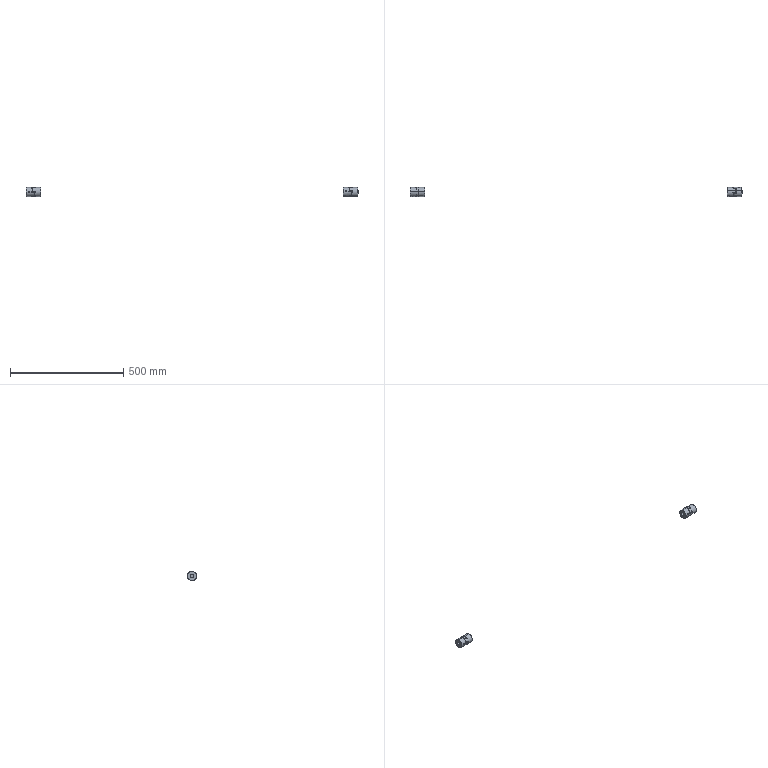Part | SolidWorks | 6 solids | 376 faces | box 1463 x 40 x 40 mm | volume 130548 mm3 | cone 176 | cylinder 160 | plane 40 | commonest cylinder face diameters 23 x70 3 x24 40 x20 4.134 x16 25 x14 16 x8